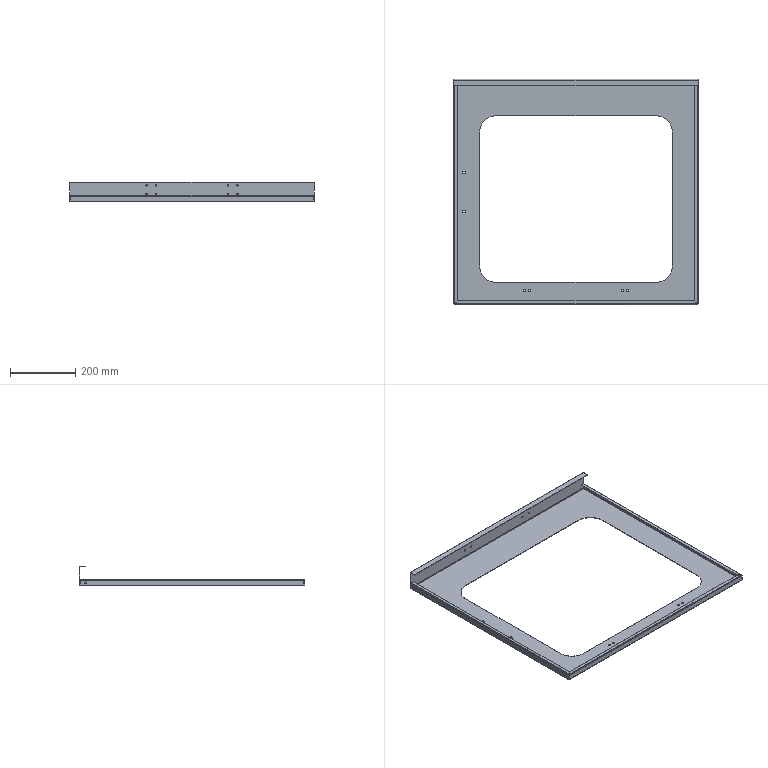Part | STEP file | Sheet metal sliding door 1 | 1 solid | 110 faces | box 750 x 690 x 61 mm | volume 498963 mm3 | plane 52 | cylinder 50 | spline 8 | commonest cylinder face diameters 4.5 x16 2 x8 5 x8 6.5 x8 8.5 x4 100 x4